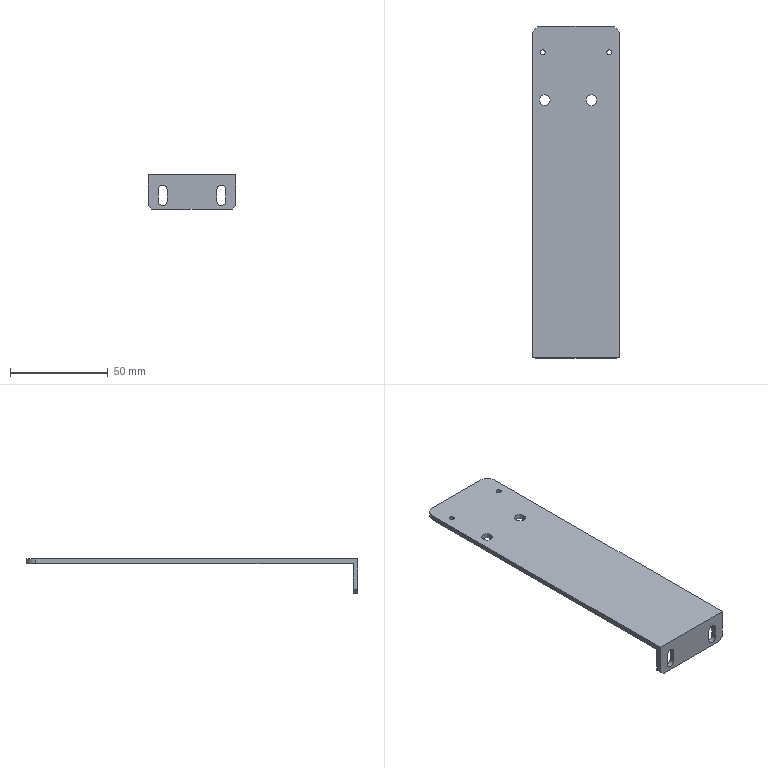Part | STEP file | PN_0108 Mount electronic clip sensor mounting plate 1 | 1 solid | 30 faces | box 45 x 170 x 17.5 mm | volume 20418 mm3 | cylinder 16 | plane 14 | commonest cylinder face diameters 4.5 x6 2.5 x4 5.5 x4 10 x2